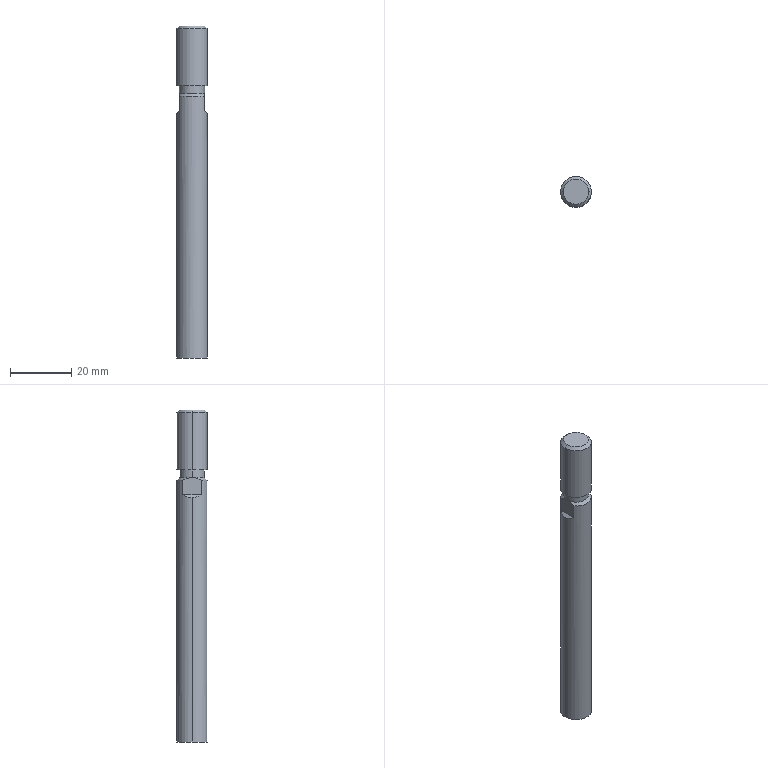Part | STEP file | 2-2 | 1 solid | 19 faces | box 10 x 10 x 108 mm | volume 8348 mm3 | plane 9 | cylinder 6 | cone 4 | commonest cylinder face diameters 10 x4 8.16 x2
STEP:
#1=CARTESIAN_POINT('',(4.,3.,4.5));
#2=VERTEX_POINT('',#1);
#3=CARTESIAN_POINT('',(5.,0.,3.5));
#4=VERTEX_POINT('',#3);
#5=CARTESIAN_POINT('',(4.,3.,4.5));
#6=CARTESIAN_POINT('',(4.655,2.127,3.845));
#7=CARTESIAN_POINT('',(5.,1.091,3.5));
#8=CARTESIAN_POINT('',(5.,0.,3.5));
#9=(BOUNDED_CURVE()B_SPLINE_CURVE(3,(#5,#6,#7,#8),.UNSPECIFIED.,.F.,.T.)B_SPLINE_CURVE_WITH_KNOTS((4,4),(5.64,6.283),.UNSPECIFIED.)CURVE()GEOMETRIC_REPRESENTATION_ITEM()RATIONAL_B_SPLINE_CURVE((1.,0.9658,0.9658,1.))REPRESENTATION_ITEM(''));
#10=EDGE_CURVE('',#2,#4,#9,.T.);
#11=ORIENTED_EDGE('',*,*,#10,.T.);
#12=CARTESIAN_POINT('',(5.,0.,-76.));
#13=VERTEX_POINT('',#12);
#14=CARTESIAN_POINT('',(5.,0.,-33.46));
#15=DIRECTION('',(0.,0.,-1.));
#16=VECTOR('',#15,1000.);
#17=LINE('',#14,#16);
#18=EDGE_CURVE('',#4,#13,#17,.T.);
#19=ORIENTED_EDGE('',*,*,#18,.T.);
#20=CARTESIAN_POINT('',(-5.,0.,-76.));
#21=VERTEX_POINT('',#20);
#22=CARTESIAN_POINT('',(0.,0.,-76.));
#23=DIRECTION('',(0.,0.,1.));
#24=DIRECTION('',(-1.,0.,0.));
#25=AXIS2_PLACEMENT_3D('',#22,#23,#24);
#26=CIRCLE('',#25,5.);
#27=EDGE_CURVE('',#13,#21,#26,.T.);
#28=ORIENTED_EDGE('',*,*,#27,.T.);
#29=CARTESIAN_POINT('',(-5.,0.,3.5));
#30=VERTEX_POINT('',#29);
#31=CARTESIAN_POINT('',(-5.,0.,-33.46));
#32=DIRECTION('',(0.,0.,-1.));
#33=VECTOR('',#32,1000.);
#34=LINE('',#31,#33);
#35=EDGE_CURVE('',#30,#21,#34,.T.);
#36=ORIENTED_EDGE('',*,*,#35,.F.);
#37=CARTESIAN_POINT('',(-4.,3.,4.5));
#38=VERTEX_POINT('',#37);
#39=CARTESIAN_POINT('',(-5.,0.,3.5));
#40=CARTESIAN_POINT('',(-5.,1.091,3.5));
#41=CARTESIAN_POINT('',(-4.655,2.127,3.845));
#42=CARTESIAN_POINT('',(-4.,3.,4.5));
#43=(BOUNDED_CURVE()B_SPLINE_CURVE(3,(#39,#40,#41,#42),.UNSPECIFIED.,.F.,.T.)B_SPLINE_CURVE_WITH_KNOTS((4,4),(0.,0.6435),.UNSPECIFIED.)CURVE()GEOMETRIC_REPRESENTATION_ITEM()RATIONAL_B_SPLINE_CURVE((1.,0.9658,0.9658,1.))REPRESENTATION_ITEM(''));
#44=EDGE_CURVE('',#30,#38,#43,.T.);
#45=ORIENTED_EDGE('',*,*,#44,.T.);
#46=CARTESIAN_POINT('',(-4.,3.,9.08));
#47=VERTEX_POINT('',#46);
#48=CARTESIAN_POINT('',(-4.,3.,-33.46));
#49=DIRECTION('',(0.,0.,1.));
#50=VECTOR('',#49,1000.);
#51=LINE('',#48,#50);
#52=EDGE_CURVE('',#38,#47,#51,.T.);
#53=ORIENTED_EDGE('',*,*,#52,.T.);
#54=CARTESIAN_POINT('',(4.,3.,9.08));
#55=VERTEX_POINT('',#54);
#56=CARTESIAN_POINT('',(0.,0.,9.08));
#57=DIRECTION('',(0.,0.,-1.));
#58=DIRECTION('',(-1.,0.,0.));
#59=AXIS2_PLACEMENT_3D('',#56,#57,#58);
#60=CIRCLE('',#59,5.);
#61=EDGE_CURVE('',#47,#55,#60,.T.);
#62=ORIENTED_EDGE('',*,*,#61,.T.);
#63=CARTESIAN_POINT('',(4.,3.,-33.46));
#64=DIRECTION('',(0.,0.,-1.));
#65=VECTOR('',#64,1000.);
#66=LINE('',#63,#65);
#67=EDGE_CURVE('',#55,#2,#66,.T.);
#68=ORIENTED_EDGE('',*,*,#67,.T.);
#69=EDGE_LOOP('',(#11,#19,#28,#36,#45,#53,#62,#68));
#70=FACE_OUTER_BOUND('',#69,.T.);
#71=CARTESIAN_POINT('',(0.,0.,-33.46));
#72=DIRECTION('',(0.,0.,-1.));
#73=DIRECTION('',(-1.,0.,0.));
#74=AXIS2_PLACEMENT_3D('',#71,#72,#73);
#75=CYLINDRICAL_SURFACE('',#74,5.);
#76=ADVANCED_FACE('',(#70),#75,.T.);
#77=CARTESIAN_POINT('',(-4.08,0.,12.5));
#78=VERTEX_POINT('',#77);
#79=CARTESIAN_POINT('',(4.08,0.,12.5));
#80=VERTEX_POINT('',#79);
#81=CARTESIAN_POINT('',(0.,0.,12.5));
#82=DIRECTION('',(0.,0.,-1.));
#83=DIRECTION('',(-1.,0.,0.));
#84=AXIS2_PLACEMENT_3D('',#81,#82,#83);
#85=CIRCLE('',#84,4.08);
#86=EDGE_CURVE('',#78,#80,#85,.T.);
#87=ORIENTED_EDGE('',*,*,#86,.T.);
#88=CARTESIAN_POINT('',(4.08,0.,10.));
#89=VERTEX_POINT('',#88);
#90=CARTESIAN_POINT('',(4.08,0.,11.25));
#91=DIRECTION('',(0.,0.,-1.));
#92=VECTOR('',#91,1000.);
#93=LINE('',#90,#92);
#94=EDGE_CURVE('',#80,#89,#93,.T.);
#95=ORIENTED_EDGE('',*,*,#94,.T.);
#96=CARTESIAN_POINT('',(4.,0.804,10.));
#97=VERTEX_POINT('',#96);
#98=CARTESIAN_POINT('',(0.,0.,10.));
#99=DIRECTION('',(0.,0.,1.));
#100=DIRECTION('',(-1.,0.,0.));
#101=AXIS2_PLACEMENT_3D('',#98,#99,#100);
#102=CIRCLE('',#101,4.08);
#103=EDGE_CURVE('',#89,#97,#102,.T.);
#104=ORIENTED_EDGE('',*,*,#103,.T.);
#105=CARTESIAN_POINT('',(-4.,0.804,10.));
#106=VERTEX_POINT('',#105);
#107=CARTESIAN_POINT('',(0.,0.,10.));
#108=DIRECTION('',(0.,0.,-1.));
#109=DIRECTION('',(0.,1.,0.));
#110=AXIS2_PLACEMENT_3D('',#107,#108,#109);
#111=CIRCLE('',#110,4.08);
#112=EDGE_CURVE('',#106,#97,#111,.T.);
#113=ORIENTED_EDGE('',*,*,#112,.F.);
#114=CARTESIAN_POINT('',(-4.08,0.,10.));
#115=VERTEX_POINT('',#114);
#116=CARTESIAN_POINT('',(0.,0.,10.));
#117=DIRECTION('',(0.,0.,1.));
#118=DIRECTION('',(-1.,0.,0.));
#119=AXIS2_PLACEMENT_3D('',#116,#117,#118);
#120=CIRCLE('',#119,4.08);
#121=EDGE_CURVE('',#106,#115,#120,.T.);
#122=ORIENTED_EDGE('',*,*,#121,.T.);
#123=CARTESIAN_POINT('',(-4.08,0.,11.25));
#124=DIRECTION('',(0.,0.,-1.));
#125=VECTOR('',#124,1000.);
#126=LINE('',#123,#125);
#127=EDGE_CURVE('',#78,#115,#126,.T.);
#128=ORIENTED_EDGE('',*,*,#127,.F.);
#129=EDGE_LOOP('',(#87,#95,#104,#113,#122,#128));
#130=FACE_OUTER_BOUND('',#129,.T.);
#131=CARTESIAN_POINT('',(0.,0.,11.25));
#132=DIRECTION('',(0.,0.,-1.));
#133=DIRECTION('',(-1.,0.,0.));
#134=AXIS2_PLACEMENT_3D('',#131,#132,#133);
#135=CYLINDRICAL_SURFACE('',#134,4.08);
#136=ADVANCED_FACE('',(#130),#135,.T.);
#137=CARTESIAN_POINT('',(-5.,0.,31.08));
#138=VERTEX_POINT('',#137);
#139=CARTESIAN_POINT('',(5.,0.,31.08));
#140=VERTEX_POINT('',#139);
#141=CARTESIAN_POINT('',(0.,0.,31.08));
#142=DIRECTION('',(0.,0.,-1.));
#143=DIRECTION('',(-1.,0.,0.));
#144=AXIS2_PLACEMENT_3D('',#141,#142,#143);
#145=CIRCLE('',#144,5.);
#146=EDGE_CURVE('',#138,#140,#145,.T.);
#147=ORIENTED_EDGE('',*,*,#146,.T.);
#148=CARTESIAN_POINT('',(5.,0.,12.5));
#149=VERTEX_POINT('',#148);
#150=CARTESIAN_POINT('',(5.,0.,21.79));
#151=DIRECTION('',(0.,0.,-1.));
#152=VECTOR('',#151,1000.);
#153=LINE('',#150,#152);
#154=EDGE_CURVE('',#140,#149,#153,.T.);
#155=ORIENTED_EDGE('',*,*,#154,.T.);
#156=CARTESIAN_POINT('',(-5.,0.,12.5));
#157=VERTEX_POINT('',#156);
#158=CARTESIAN_POINT('',(0.,0.,12.5));
#159=DIRECTION('',(0.,0.,-1.));
#160=DIRECTION('',(-1.,0.,0.));
#161=AXIS2_PLACEMENT_3D('',#158,#159,#160);
#162=CIRCLE('',#161,5.);
#163=EDGE_CURVE('',#157,#149,#162,.T.);
#164=ORIENTED_EDGE('',*,*,#163,.F.);
#165=CARTESIAN_POINT('',(-5.,0.,21.79));
#166=DIRECTION('',(0.,0.,-1.));
#167=VECTOR('',#166,1000.);
#168=LINE('',#165,#167);
#169=EDGE_CURVE('',#138,#157,#168,.T.);
#170=ORIENTED_EDGE('',*,*,#169,.F.);
#171=EDGE_LOOP('',(#147,#155,#164,#170));
#172=FACE_OUTER_BOUND('',#171,.T.);
#173=CARTESIAN_POINT('',(0.,0.,21.79));
#174=DIRECTION('',(0.,0.,-1.));
#175=DIRECTION('',(-1.,0.,0.));
#176=AXIS2_PLACEMENT_3D('',#173,#174,#175);
#177=CYLINDRICAL_SURFACE('',#176,5.);
#178=ADVANCED_FACE('',(#172),#177,.T.);
#179=CARTESIAN_POINT('',(-4.08,0.,32.));
#180=VERTEX_POINT('',#179);
#181=CARTESIAN_POINT('',(4.08,0.,32.));
#182=VERTEX_POINT('',#181);
#183=CARTESIAN_POINT('',(0.,0.,32.));
#184=DIRECTION('',(0.,0.,-1.));
#185=DIRECTION('',(-1.,0.,0.));
#186=AXIS2_PLACEMENT_3D('',#183,#184,#185);
#187=CIRCLE('',#186,4.08);
#188=EDGE_CURVE('',#180,#182,#187,.T.);
#189=ORIENTED_EDGE('',*,*,#188,.T.);
#190=CARTESIAN_POINT('',(5.,0.,31.08));
#191=DIRECTION('',(0.7071,0.,-0.7071));
#192=VECTOR('',#191,1000.);
#193=LINE('',#190,#192);
#194=EDGE_CURVE('',#182,#140,#193,.T.);
#195=ORIENTED_EDGE('',*,*,#194,.T.);
#196=ORIENTED_EDGE('',*,*,#146,.F.);
#197=CARTESIAN_POINT('',(-5.,0.,31.08));
#198=DIRECTION('',(-0.7071,0.,-0.7071));
#199=VECTOR('',#198,1000.);
#200=LINE('',#197,#199);
#201=EDGE_CURVE('',#180,#138,#200,.T.);
#202=ORIENTED_EDGE('',*,*,#201,.F.);
#203=EDGE_LOOP('',(#189,#195,#196,#202));
#204=FACE_OUTER_BOUND('',#203,.T.);
#205=CARTESIAN_POINT('',(0.,0.,31.08));
#206=DIRECTION('',(0.,0.,-1.));
#207=DIRECTION('',(-1.,0.,0.));
#208=AXIS2_PLACEMENT_3D('',#205,#206,#207);
#209=CONICAL_SURFACE('',#208,5.,0.7854);
#210=ADVANCED_FACE('',(#204),#209,.T.);
#211=ORIENTED_EDGE('',*,*,#18,.F.);
#212=CARTESIAN_POINT('',(4.,-3.,4.5));
#213=VERTEX_POINT('',#212);
#214=CARTESIAN_POINT('',(5.,0.,3.5));
#215=CARTESIAN_POINT('',(5.,-1.091,3.5));
#216=CARTESIAN_POINT('',(4.655,-2.127,3.845));
#217=CARTESIAN_POINT('',(4.,-3.,4.5));
#218=(BOUNDED_CURVE()B_SPLINE_CURVE(3,(#214,#215,#216,#217),.UNSPECIFIED.,.F.,.T.)B_SPLINE_CURVE_WITH_KNOTS((4,4),(0.,0.6435),.UNSPECIFIED.)CURVE()GEOMETRIC_REPRESENTATION_ITEM()RATIONAL_B_SPLINE_CURVE((1.,0.9658,0.9658,1.))REPRESENTATION_ITEM(''));
#219=EDGE_CURVE('',#4,#213,#218,.T.);
#220=ORIENTED_EDGE('',*,*,#219,.T.);
#221=CARTESIAN_POINT('',(4.,-3.,9.08));
#222=VERTEX_POINT('',#221);
#223=CARTESIAN_POINT('',(4.,-3.,-33.46));
#224=DIRECTION('',(0.,0.,1.));
#225=VECTOR('',#224,1000.);
#226=LINE('',#223,#225);
#227=EDGE_CURVE('',#213,#222,#226,.T.);
#228=ORIENTED_EDGE('',*,*,#227,.T.);
#229=CARTESIAN_POINT('',(-4.,-3.,9.08));
#230=VERTEX_POINT('',#229);
#231=CARTESIAN_POINT('',(0.,0.,9.08));
#232=DIRECTION('',(0.,0.,-1.));
#233=DIRECTION('',(-1.,0.,0.));
#234=AXIS2_PLACEMENT_3D('',#231,#232,#233);
#235=CIRCLE('',#234,5.);
#236=EDGE_CURVE('',#222,#230,#235,.T.);
#237=ORIENTED_EDGE('',*,*,#236,.T.);
#238=CARTESIAN_POINT('',(-4.,-3.,4.5));
#239=VERTEX_POINT('',#238);
#240=CARTESIAN_POINT('',(-4.,-3.,-33.46));
#241=DIRECTION('',(0.,0.,-1.));
#242=VECTOR('',#241,1000.);
#243=LINE('',#240,#242);
#244=EDGE_CURVE('',#230,#239,#243,.T.);
#245=ORIENTED_EDGE('',*,*,#244,.T.);
#246=CARTESIAN_POINT('',(-4.,-3.,4.5));
#247=CARTESIAN_POINT('',(-4.655,-2.127,3.845));
#248=CARTESIAN_POINT('',(-5.,-1.091,3.5));
#249=CARTESIAN_POINT('',(-5.,0.,3.5));
#250=(BOUNDED_CURVE()B_SPLINE_CURVE(3,(#246,#247,#248,#249),.UNSPECIFIED.,.F.,.T.)B_SPLINE_CURVE_WITH_KNOTS((4,4),(5.64,6.283),.UNSPECIFIED.)CURVE()GEOMETRIC_REPRESENTATION_ITEM()RATIONAL_B_SPLINE_CURVE((1.,0.9658,0.9658,1.))REPRESENTATION_ITEM(''));
#251=EDGE_CURVE('',#239,#30,#250,.T.);
#252=ORIENTED_EDGE('',*,*,#251,.T.);
#253=ORIENTED_EDGE('',*,*,#35,.T.);
#254=CARTESIAN_POINT('',(0.,0.,-76.));
#255=DIRECTION('',(0.,0.,1.));
#256=DIRECTION('',(-1.,0.,0.));
#257=AXIS2_PLACEMENT_3D('',#254,#255,#256);
#258=CIRCLE('',#257,5.);
#259=EDGE_CURVE('',#21,#13,#258,.T.);
#260=ORIENTED_EDGE('',*,*,#259,.T.);
#261=EDGE_LOOP('',(#211,#220,#228,#237,#245,#252,#253,#260));
#262=FACE_OUTER_BOUND('',#261,.T.);
#263=CARTESIAN_POINT('',(0.,0.,-33.46));
#264=DIRECTION('',(0.,0.,-1.));
#265=DIRECTION('',(-1.,0.,0.));
#266=AXIS2_PLACEMENT_3D('',#263,#264,#265);
#267=CYLINDRICAL_SURFACE('',#266,5.);
#268=ADVANCED_FACE('',(#262),#267,.T.);
#269=ORIENTED_EDGE('',*,*,#259,.F.);
#270=ORIENTED_EDGE('',*,*,#27,.F.);
#271=EDGE_LOOP('',(#269,#270));
#272=FACE_OUTER_BOUND('',#271,.T.);
#273=CARTESIAN_POINT('',(0.,2.5,-76.));
#274=DIRECTION('',(0.,0.,-1.));
#275=DIRECTION('',(-1.,0.,0.));
#276=AXIS2_PLACEMENT_3D('',#273,#274,#275);
#277=PLANE('',#276);
#278=ADVANCED_FACE('',(#272),#277,.T.);
#279=CARTESIAN_POINT('',(4.,-0.804,10.));
#280=VERTEX_POINT('',#279);
#281=CARTESIAN_POINT('',(4.,-3.,9.08));
#282=CARTESIAN_POINT('',(4.,-2.656,9.286));
#283=CARTESIAN_POINT('',(4.,-2.305,9.475));
#284=CARTESIAN_POINT('',(4.,-1.578,9.793));
#285=CARTESIAN_POINT('',(4.,-1.201,9.922));
#286=CARTESIAN_POINT('',(4.,-0.804,10.));
#287=B_SPLINE_CURVE_WITH_KNOTS('',3,(#281,#282,#283,#284,#285,#286),.UNSPECIFIED.,.F.,.F.,(4,2,4),(0.,0.00119,0.002381),.UNSPECIFIED.);
#288=EDGE_CURVE('',#222,#280,#287,.T.);
#289=ORIENTED_EDGE('',*,*,#288,.T.);
#290=CARTESIAN_POINT('',(-4.,-0.804,10.));
#291=VERTEX_POINT('',#290);
#292=CARTESIAN_POINT('',(0.,0.,10.));
#293=DIRECTION('',(0.,0.,-1.));
#294=DIRECTION('',(0.,1.,0.));
#295=AXIS2_PLACEMENT_3D('',#292,#293,#294);
#296=CIRCLE('',#295,4.08);
#297=EDGE_CURVE('',#280,#291,#296,.T.);
#298=ORIENTED_EDGE('',*,*,#297,.T.);
#299=CARTESIAN_POINT('',(-4.,-0.804,10.));
#300=CARTESIAN_POINT('',(-4.,-1.199,9.922));
#301=CARTESIAN_POINT('',(-4.,-1.575,9.794));
#302=CARTESIAN_POINT('',(-4.,-2.303,9.476));
#303=CARTESIAN_POINT('',(-4.,-2.657,9.286));
#304=CARTESIAN_POINT('',(-4.,-3.,9.08));
#305=B_SPLINE_CURVE_WITH_KNOTS('',3,(#299,#300,#301,#302,#303,#304),.UNSPECIFIED.,.F.,.F.,(4,2,4),(0.,0.001191,0.002382),.UNSPECIFIED.);
#306=EDGE_CURVE('',#291,#230,#305,.T.);
#307=ORIENTED_EDGE('',*,*,#306,.T.);
#308=ORIENTED_EDGE('',*,*,#236,.F.);
#309=EDGE_LOOP('',(#289,#298,#307,#308));
#310=FACE_OUTER_BOUND('',#309,.T.);
#311=CARTESIAN_POINT('',(0.,0.,9.08));
#312=DIRECTION('',(0.,0.,-1.));
#313=DIRECTION('',(-1.,0.,0.));
#314=AXIS2_PLACEMENT_3D('',#311,#312,#313);
#315=CONICAL_SURFACE('',#314,5.,0.7854);
#316=ADVANCED_FACE('',(#310),#315,.T.);
#317=ORIENTED_EDGE('',*,*,#227,.F.);
#318=CARTESIAN_POINT('',(4.,10.,4.5));
#319=DIRECTION('',(0.,-1.,0.));
#320=VECTOR('',#319,1000.);
#321=LINE('',#318,#320);
#322=EDGE_CURVE('',#2,#213,#321,.T.);
#323=ORIENTED_EDGE('',*,*,#322,.F.);
#324=ORIENTED_EDGE('',*,*,#67,.F.);
#325=CARTESIAN_POINT('',(4.,0.804,10.));
#326=CARTESIAN_POINT('',(4.,1.199,9.922));
#327=CARTESIAN_POINT('',(4.,1.575,9.794));
#328=CARTESIAN_POINT('',(4.,2.303,9.476));
#329=CARTESIAN_POINT('',(4.,2.657,9.286));
#330=CARTESIAN_POINT('',(4.,3.,9.08));
#331=B_SPLINE_CURVE_WITH_KNOTS('',3,(#325,#326,#327,#328,#329,#330),.UNSPECIFIED.,.F.,.F.,(4,2,4),(0.,0.001191,0.002382),.UNSPECIFIED.);
#332=EDGE_CURVE('',#97,#55,#331,.T.);
#333=ORIENTED_EDGE('',*,*,#332,.F.);
#334=CARTESIAN_POINT('',(4.,10.,10.));
#335=DIRECTION('',(0.,1.,0.));
#336=VECTOR('',#335,1000.);
#337=LINE('',#334,#336);
#338=EDGE_CURVE('',#280,#97,#337,.T.);
#339=ORIENTED_EDGE('',*,*,#338,.F.);
#340=ORIENTED_EDGE('',*,*,#288,.F.);
#341=EDGE_LOOP('',(#317,#323,#324,#333,#339,#340));
#342=FACE_OUTER_BOUND('',#341,.T.);
#343=CARTESIAN_POINT('',(4.,10.,4.5));
#344=DIRECTION('',(-1.,0.,0.));
#345=DIRECTION('',(0.,0.,1.));
#346=AXIS2_PLACEMENT_3D('',#343,#344,#345);
#347=PLANE('',#346);
#348=ADVANCED_FACE('',(#342),#347,.F.);
#349=ORIENTED_EDGE('',*,*,#322,.T.);
#350=ORIENTED_EDGE('',*,*,#219,.F.);
#351=ORIENTED_EDGE('',*,*,#10,.F.);
#352=EDGE_LOOP('',(#349,#350,#351));
#353=FACE_OUTER_BOUND('',#352,.T.);
#354=CARTESIAN_POINT('',(5.,10.,3.5));
#355=DIRECTION('',(-0.7071,0.,-0.7071));
#356=DIRECTION('',(-0.7071,0.,0.7071));
#357=AXIS2_PLACEMENT_3D('',#354,#355,#356);
#358=PLANE('',#357);
#359=ADVANCED_FACE('',(#353),#358,.F.);
#360=ORIENTED_EDGE('',*,*,#332,.T.);
#361=ORIENTED_EDGE('',*,*,#61,.F.);
#362=CARTESIAN_POINT('',(-4.,3.,9.08));
#363=CARTESIAN_POINT('',(-4.,2.656,9.286));
#364=CARTESIAN_POINT('',(-4.,2.305,9.475));
#365=CARTESIAN_POINT('',(-4.,1.578,9.793));
#366=CARTESIAN_POINT('',(-4.,1.201,9.922));
#367=CARTESIAN_POINT('',(-4.,0.804,10.));
#368=B_SPLINE_CURVE_WITH_KNOTS('',3,(#362,#363,#364,#365,#366,#367),.UNSPECIFIED.,.F.,.F.,(4,2,4),(0.,0.00119,0.002381),.UNSPECIFIED.);
#369=EDGE_CURVE('',#47,#106,#368,.T.);
#370=ORIENTED_EDGE('',*,*,#369,.T.);
#371=ORIENTED_EDGE('',*,*,#112,.T.);
#372=EDGE_LOOP('',(#360,#361,#370,#371));
#373=FACE_OUTER_BOUND('',#372,.T.);
#374=CARTESIAN_POINT('',(0.,0.,9.08));
#375=DIRECTION('',(0.,0.,-1.));
#376=DIRECTION('',(-1.,0.,0.));
#377=AXIS2_PLACEMENT_3D('',#374,#375,#376);
#378=CONICAL_SURFACE('',#377,5.,0.7854);
#379=ADVANCED_FACE('',(#373),#378,.T.);
#380=CARTESIAN_POINT('',(-4.,10.,10.));
#381=DIRECTION('',(0.,-1.,0.));
#382=VECTOR('',#381,1000.);
#383=LINE('',#380,#382);
#384=EDGE_CURVE('',#106,#291,#383,.T.);
#385=ORIENTED_EDGE('',*,*,#384,.F.);
#386=ORIENTED_EDGE('',*,*,#369,.F.);
#387=ORIENTED_EDGE('',*,*,#52,.F.);
#388=CARTESIAN_POINT('',(-4.,10.,4.5));
#389=DIRECTION('',(0.,1.,0.));
#390=VECTOR('',#389,1000.);
#391=LINE('',#388,#390);
#392=EDGE_CURVE('',#239,#38,#391,.T.);
#393=ORIENTED_EDGE('',*,*,#392,.F.);
#394=ORIENTED_EDGE('',*,*,#244,.F.);
#395=ORIENTED_EDGE('',*,*,#306,.F.);
#396=EDGE_LOOP('',(#385,#386,#387,#393,#394,#395));
#397=FACE_OUTER_BOUND('',#396,.T.);
#398=CARTESIAN_POINT('',(-4.,10.,10.));
#399=DIRECTION('',(1.,0.,0.));
#400=DIRECTION('',(0.,0.,-1.));
#401=AXIS2_PLACEMENT_3D('',#398,#399,#400);
#402=PLANE('',#401);
#403=ADVANCED_FACE('',(#397),#402,.F.);
#404=ORIENTED_EDGE('',*,*,#392,.T.);
#405=ORIENTED_EDGE('',*,*,#44,.F.);
#406=ORIENTED_EDGE('',*,*,#251,.F.);
#407=EDGE_LOOP('',(#404,#405,#406));
#408=FACE_OUTER_BOUND('',#407,.T.);
#409=CARTESIAN_POINT('',(-4.,10.,4.5));
#410=DIRECTION('',(0.7071,0.,-0.7071));
#411=DIRECTION('',(-0.7071,0.,-0.7071));
#412=AXIS2_PLACEMENT_3D('',#409,#410,#411);
#413=PLANE('',#412);
#414=ADVANCED_FACE('',(#408),#413,.F.);
#415=ORIENTED_EDGE('',*,*,#94,.F.);
#416=CARTESIAN_POINT('',(0.,0.,12.5));
#417=DIRECTION('',(0.,0.,-1.));
#418=DIRECTION('',(-1.,0.,0.));
#419=AXIS2_PLACEMENT_3D('',#416,#417,#418);
#420=CIRCLE('',#419,4.08);
#421=EDGE_CURVE('',#80,#78,#420,.T.);
#422=ORIENTED_EDGE('',*,*,#421,.T.);
#423=ORIENTED_EDGE('',*,*,#127,.T.);
#424=CARTESIAN_POINT('',(0.,0.,10.));
#425=DIRECTION('',(0.,0.,1.));
#426=DIRECTION('',(-1.,0.,0.));
#427=AXIS2_PLACEMENT_3D('',#424,#425,#426);
#428=CIRCLE('',#427,4.08);
#429=EDGE_CURVE('',#115,#291,#428,.T.);
#430=ORIENTED_EDGE('',*,*,#429,.T.);
#431=ORIENTED_EDGE('',*,*,#297,.F.);
#432=CARTESIAN_POINT('',(0.,0.,10.));
#433=DIRECTION('',(0.,0.,1.));
#434=DIRECTION('',(-1.,0.,0.));
#435=AXIS2_PLACEMENT_3D('',#432,#433,#434);
#436=CIRCLE('',#435,4.08);
#437=EDGE_CURVE('',#280,#89,#436,.T.);
#438=ORIENTED_EDGE('',*,*,#437,.T.);
#439=EDGE_LOOP('',(#415,#422,#423,#430,#431,#438));
#440=FACE_OUTER_BOUND('',#439,.T.);
#441=CARTESIAN_POINT('',(0.,0.,11.25));
#442=DIRECTION('',(0.,0.,-1.));
#443=DIRECTION('',(-1.,0.,0.));
#444=AXIS2_PLACEMENT_3D('',#441,#442,#443);
#445=CYLINDRICAL_SURFACE('',#444,4.08);
#446=ADVANCED_FACE('',(#440),#445,.T.);
#447=ORIENTED_EDGE('',*,*,#338,.T.);
#448=ORIENTED_EDGE('',*,*,#103,.F.);
#449=ORIENTED_EDGE('',*,*,#437,.F.);
#450=EDGE_LOOP('',(#447,#448,#449));
#451=FACE_OUTER_BOUND('',#450,.T.);
#452=CARTESIAN_POINT('',(4.,10.,10.));
#453=DIRECTION('',(0.,0.,1.));
#454=DIRECTION('',(1.,0.,0.));
#455=AXIS2_PLACEMENT_3D('',#452,#453,#454);
#456=PLANE('',#455);
#457=ADVANCED_FACE('',(#451),#456,.F.);
#458=ORIENTED_EDGE('',*,*,#384,.T.);
#459=ORIENTED_EDGE('',*,*,#429,.F.);
#460=ORIENTED_EDGE('',*,*,#121,.F.);
#461=EDGE_LOOP('',(#458,#459,#460));
#462=FACE_OUTER_BOUND('',#461,.T.);
#463=CARTESIAN_POINT('',(-7.,10.,10.));
#464=DIRECTION('',(0.,0.,1.));
#465=DIRECTION('',(1.,0.,0.));
#466=AXIS2_PLACEMENT_3D('',#463,#464,#465);
#467=PLANE('',#466);
#468=ADVANCED_FACE('',(#462),#467,.F.);
#469=ORIENTED_EDGE('',*,*,#86,.F.);
#470=ORIENTED_EDGE('',*,*,#421,.F.);
#471=EDGE_LOOP('',(#469,#470));
#472=FACE_BOUND('',#471,.T.);
#473=ORIENTED_EDGE('',*,*,#163,.T.);
#474=CARTESIAN_POINT('',(0.,0.,12.5));
#475=DIRECTION('',(0.,0.,-1.));
#476=DIRECTION('',(-1.,0.,0.));
#477=AXIS2_PLACEMENT_3D('',#474,#475,#476);
#478=CIRCLE('',#477,5.);
#479=EDGE_CURVE('',#149,#157,#478,.T.);
#480=ORIENTED_EDGE('',*,*,#479,.T.);
#481=EDGE_LOOP('',(#473,#480));
#482=FACE_OUTER_BOUND('',#481,.T.);
#483=CARTESIAN_POINT('',(0.,4.54,12.5));
#484=DIRECTION('',(0.,0.,-1.));
#485=DIRECTION('',(-1.,0.,0.));
#486=AXIS2_PLACEMENT_3D('',#483,#484,#485);
#487=PLANE('',#486);
#488=ADVANCED_FACE('',(#472,#482),#487,.T.);
#489=ORIENTED_EDGE('',*,*,#154,.F.);
#490=CARTESIAN_POINT('',(0.,0.,31.08));
#491=DIRECTION('',(0.,0.,-1.));
#492=DIRECTION('',(-1.,0.,0.));
#493=AXIS2_PLACEMENT_3D('',#490,#491,#492);
#494=CIRCLE('',#493,5.);
#495=EDGE_CURVE('',#140,#138,#494,.T.);
#496=ORIENTED_EDGE('',*,*,#495,.T.);
#497=ORIENTED_EDGE('',*,*,#169,.T.);
#498=ORIENTED_EDGE('',*,*,#479,.F.);
#499=EDGE_LOOP('',(#489,#496,#497,#498));
#500=FACE_OUTER_BOUND('',#499,.T.);
#501=CARTESIAN_POINT('',(0.,0.,21.79));
#502=DIRECTION('',(0.,0.,-1.));
#503=DIRECTION('',(-1.,0.,0.));
#504=AXIS2_PLACEMENT_3D('',#501,#502,#503);
#505=CYLINDRICAL_SURFACE('',#504,5.);
#506=ADVANCED_FACE('',(#500),#505,.T.);
#507=ORIENTED_EDGE('',*,*,#194,.F.);
#508=CARTESIAN_POINT('',(0.,0.,32.));
#509=DIRECTION('',(0.,0.,-1.));
#510=DIRECTION('',(-1.,0.,0.));
#511=AXIS2_PLACEMENT_3D('',#508,#509,#510);
#512=CIRCLE('',#511,4.08);
#513=EDGE_CURVE('',#182,#180,#512,.T.);
#514=ORIENTED_EDGE('',*,*,#513,.T.);
#515=ORIENTED_EDGE('',*,*,#201,.T.);
#516=ORIENTED_EDGE('',*,*,#495,.F.);
#517=EDGE_LOOP('',(#507,#514,#515,#516));
#518=FACE_OUTER_BOUND('',#517,.T.);
#519=CARTESIAN_POINT('',(0.,0.,31.08));
#520=DIRECTION('',(0.,0.,-1.));
#521=DIRECTION('',(-1.,0.,0.));
#522=AXIS2_PLACEMENT_3D('',#519,#520,#521);
#523=CONICAL_SURFACE('',#522,5.,0.7854);
#524=ADVANCED_FACE('',(#518),#523,.T.);
#525=ORIENTED_EDGE('',*,*,#188,.F.);
#526=ORIENTED_EDGE('',*,*,#513,.F.);
#527=EDGE_LOOP('',(#525,#526));
#528=FACE_OUTER_BOUND('',#527,.T.);
#529=CARTESIAN_POINT('',(0.,2.04,32.));
#530=DIRECTION('',(0.,0.,1.));
#531=DIRECTION('',(1.,0.,0.));
#532=AXIS2_PLACEMENT_3D('',#529,#530,#531);
#533=PLANE('',#532);
#534=ADVANCED_FACE('',(#528),#533,.T.);
#535=CLOSED_SHELL('',(#76,#136,#178,#210,#268,#278,#316,#348,#359,#379,#403,#414,#446,#457,#468,#488,#506,#524,#534));
#536=MANIFOLD_SOLID_BREP('',#535);
#537=CARTESIAN_POINT('',(0.,0.,0.));
#538=DIRECTION('',(0.,0.,1.));
#539=DIRECTION('',(1.,0.,0.));
#540=AXIS2_PLACEMENT_3D('',#537,#538,#539);
#541=(LENGTH_UNIT()NAMED_UNIT(*)SI_UNIT(.MILLI.,.METRE.));
#542=UNCERTAINTY_MEASURE_WITH_UNIT(LENGTH_MEASURE(0.00001),#541,'','');
#543=(NAMED_UNIT(*)PLANE_ANGLE_UNIT()SI_UNIT($,.RADIAN.));
#544=(NAMED_UNIT(*)SI_UNIT($,.STERADIAN.)SOLID_ANGLE_UNIT());
#545=(GEOMETRIC_REPRESENTATION_CONTEXT(3)GLOBAL_UNCERTAINTY_ASSIGNED_CONTEXT((#542))GLOBAL_UNIT_ASSIGNED_CONTEXT((#541,#543,#544))REPRESENTATION_CONTEXT('',''));
#546=ADVANCED_BREP_SHAPE_REPRESENTATION('',(#536,#540),#545);